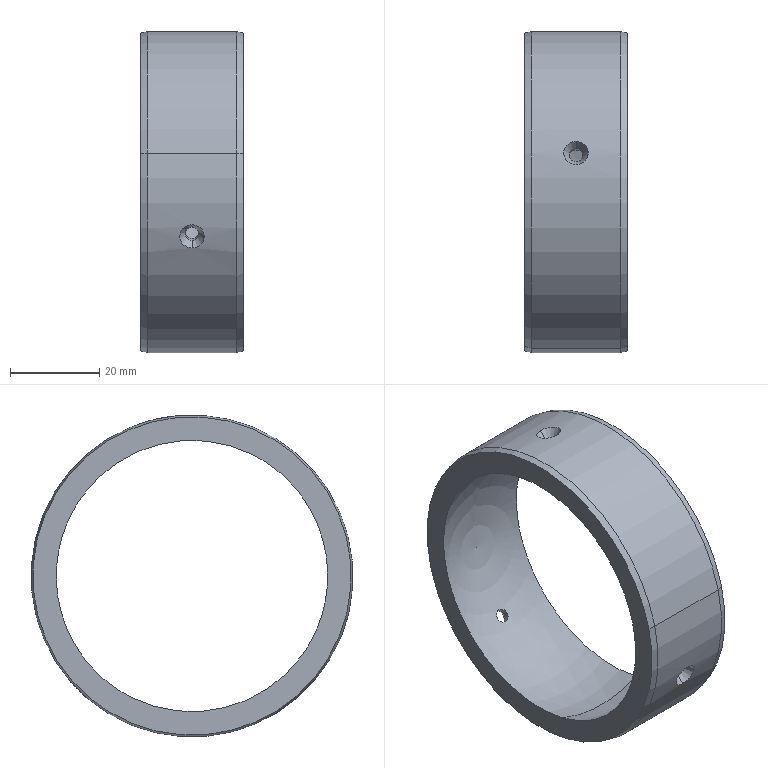Part | SolidWorks | features BaseBody 1 | 1 solid | 22 faces | box 23 x 72 x 72 mm | volume 20485 mm3 | cone 10 | cylinder 8 | sphere 2 | plane 2 | commonest cylinder face diameters 3 x6 72 x2
STEP:
#1=CARTESIAN_POINT('',(272.,34.546,-8.591));
#2=VERTEX_POINT('',#1);
#3=CARTESIAN_POINT('',(272.,-34.546,8.591));
#4=VERTEX_POINT('',#3);
#5=CARTESIAN_POINT('',(272.,0.,0.));
#6=DIRECTION('',(1.,0.,0.));
#7=DIRECTION('',(0.,0.9704,-0.2413));
#8=AXIS2_PLACEMENT_3D('',#5,#6,#7);
#9=CIRCLE('',#8,35.598);
#10=EDGE_CURVE('',#2,#4,#9,.T.);
#11=ORIENTED_EDGE('',*,*,#10,.F.);
#12=CARTESIAN_POINT('',(270.5,34.936,-8.688));
#13=VERTEX_POINT('',#12);
#14=CARTESIAN_POINT('',(272.,34.546,-8.591));
#15=DIRECTION('',(-0.9659,0.2512,-0.06246));
#16=VECTOR('',#15,1000.);
#17=LINE('',#14,#16);
#18=EDGE_CURVE('',#2,#13,#17,.T.);
#19=ORIENTED_EDGE('',*,*,#18,.T.);
#20=CARTESIAN_POINT('',(270.5,-34.936,8.688));
#21=VERTEX_POINT('',#20);
#22=CARTESIAN_POINT('',(270.5,0.,0.));
#23=DIRECTION('',(-1.,0.,0.));
#24=DIRECTION('',(0.,0.9704,-0.2413));
#25=AXIS2_PLACEMENT_3D('',#22,#23,#24);
#26=CIRCLE('',#25,36.);
#27=EDGE_CURVE('',#21,#13,#26,.T.);
#28=ORIENTED_EDGE('',*,*,#27,.F.);
#29=CARTESIAN_POINT('',(272.,-34.546,8.591));
#30=DIRECTION('',(-0.9659,-0.2512,0.06246));
#31=VECTOR('',#30,1000.);
#32=LINE('',#29,#31);
#33=EDGE_CURVE('',#4,#21,#32,.T.);
#34=ORIENTED_EDGE('',*,*,#33,.F.);
#35=EDGE_LOOP('',(#11,#19,#28,#34));
#36=FACE_OUTER_BOUND('',#35,.T.);
#37=CARTESIAN_POINT('',(272.,0.,0.));
#38=DIRECTION('',(-1.,0.,0.));
#39=DIRECTION('',(0.,-0.9704,0.2413));
#40=AXIS2_PLACEMENT_3D('',#37,#38,#39);
#41=CONICAL_SURFACE('',#40,35.598,0.2618);
#42=ADVANCED_FACE('',(#36),#41,.T.);
#43=CARTESIAN_POINT('',(249.,-34.546,8.591));
#44=VERTEX_POINT('',#43);
#45=CARTESIAN_POINT('',(249.,34.546,-8.591));
#46=VERTEX_POINT('',#45);
#47=CARTESIAN_POINT('',(249.,0.,0.));
#48=DIRECTION('',(-1.,0.,0.));
#49=DIRECTION('',(0.,-0.9704,0.2413));
#50=AXIS2_PLACEMENT_3D('',#47,#48,#49);
#51=CIRCLE('',#50,35.598);
#52=EDGE_CURVE('',#44,#46,#51,.T.);
#53=ORIENTED_EDGE('',*,*,#52,.F.);
#54=CARTESIAN_POINT('',(250.5,-34.936,8.688));
#55=VERTEX_POINT('',#54);
#56=CARTESIAN_POINT('',(250.5,-34.936,8.688));
#57=DIRECTION('',(0.9659,-0.2512,0.06246));
#58=VECTOR('',#57,1000.);
#59=LINE('',#56,#58);
#60=EDGE_CURVE('',#44,#55,#59,.T.);
#61=ORIENTED_EDGE('',*,*,#60,.T.);
#62=CARTESIAN_POINT('',(250.5,34.936,-8.688));
#63=VERTEX_POINT('',#62);
#64=CARTESIAN_POINT('',(250.5,0.,0.));
#65=DIRECTION('',(1.,0.,0.));
#66=DIRECTION('',(0.,-0.9704,0.2413));
#67=AXIS2_PLACEMENT_3D('',#64,#65,#66);
#68=CIRCLE('',#67,36.);
#69=EDGE_CURVE('',#63,#55,#68,.T.);
#70=ORIENTED_EDGE('',*,*,#69,.F.);
#71=CARTESIAN_POINT('',(250.5,34.936,-8.688));
#72=DIRECTION('',(0.9659,0.2512,-0.06246));
#73=VECTOR('',#72,1000.);
#74=LINE('',#71,#73);
#75=EDGE_CURVE('',#46,#63,#74,.T.);
#76=ORIENTED_EDGE('',*,*,#75,.F.);
#77=EDGE_LOOP('',(#53,#61,#70,#76));
#78=FACE_OUTER_BOUND('',#77,.T.);
#79=CARTESIAN_POINT('',(250.5,0.,0.));
#80=DIRECTION('',(1.,0.,0.));
#81=DIRECTION('',(0.,0.9704,-0.2413));
#82=AXIS2_PLACEMENT_3D('',#79,#80,#81);
#83=CONICAL_SURFACE('',#82,36.,0.2618);
#84=ADVANCED_FACE('',(#78),#83,.T.);
#85=CARTESIAN_POINT('',(260.5,-32.933,-7.904));
#86=VERTEX_POINT('',#85);
#87=CARTESIAN_POINT('',(260.5,-32.104,-10.787));
#88=VERTEX_POINT('',#87);
#89=CARTESIAN_POINT('',(260.5,-32.519,-9.346));
#90=DIRECTION('',(0.,0.9611,0.2762));
#91=DIRECTION('',(0.,0.2762,-0.9611));
#92=AXIS2_PLACEMENT_3D('',#89,#90,#91);
#93=CIRCLE('',#92,1.5);
#94=EDGE_CURVE('',#86,#88,#93,.T.);
#95=ORIENTED_EDGE('',*,*,#94,.T.);
#96=CARTESIAN_POINT('',(260.5,-33.759,-12.503));
#97=VERTEX_POINT('',#96);
#98=CARTESIAN_POINT('',(260.5,-33.84,-12.587));
#99=DIRECTION('',(0.,-0.6942,-0.7198));
#100=VECTOR('',#99,1000.);
#101=LINE('',#98,#100);
#102=EDGE_CURVE('',#88,#97,#101,.T.);
#103=ORIENTED_EDGE('',*,*,#102,.T.);
#104=CARTESIAN_POINT('',(260.5,-35.246,-7.329));
#105=VERTEX_POINT('',#104);
#106=CARTESIAN_POINT('',(260.5,-35.246,-7.329));
#107=CARTESIAN_POINT('',(260.68,-35.246,-7.329));
#108=CARTESIAN_POINT('',(260.856,-35.243,-7.345));
#109=CARTESIAN_POINT('',(261.204,-35.229,-7.411));
#110=CARTESIAN_POINT('',(261.378,-35.218,-7.461));
#111=CARTESIAN_POINT('',(261.709,-35.191,-7.591));
#112=CARTESIAN_POINT('',(261.866,-35.173,-7.671));
#113=CARTESIAN_POINT('',(262.164,-35.132,-7.86));
#114=CARTESIAN_POINT('',(262.306,-35.107,-7.97));
#115=CARTESIAN_POINT('',(262.561,-35.051,-8.211));
#116=CARTESIAN_POINT('',(262.676,-35.02,-8.342));
#117=CARTESIAN_POINT('',(262.879,-34.951,-8.628));
#118=CARTESIAN_POINT('',(262.966,-34.913,-8.781));
#119=CARTESIAN_POINT('',(263.175,-34.792,-9.254));
#120=CARTESIAN_POINT('',(263.25,-34.698,-9.6));
#121=CARTESIAN_POINT('',(263.25,-34.551,-10.111));
#122=CARTESIAN_POINT('',(263.232,-34.5,-10.284));
#123=CARTESIAN_POINT('',(263.161,-34.399,-10.618));
#124=CARTESIAN_POINT('',(263.108,-34.349,-10.78));
#125=CARTESIAN_POINT('',(262.968,-34.249,-11.092));
#126=CARTESIAN_POINT('',(262.88,-34.2,-11.243));
#127=CARTESIAN_POINT('',(262.679,-34.107,-11.52));
#128=CARTESIAN_POINT('',(262.564,-34.063,-11.649));
#129=CARTESIAN_POINT('',(262.178,-33.941,-12.004));
#130=CARTESIAN_POINT('',(261.871,-33.874,-12.19));
#131=CARTESIAN_POINT('',(261.378,-33.806,-12.376));
#132=CARTESIAN_POINT('',(261.205,-33.788,-12.424));
#133=CARTESIAN_POINT('',(260.854,-33.765,-12.487));
#134=CARTESIAN_POINT('',(260.678,-33.759,-12.503));
#135=CARTESIAN_POINT('',(260.5,-33.759,-12.503));
#136=B_SPLINE_CURVE_WITH_KNOTS('',3,(#106,#107,#108,#109,#110,#111,#112,#113,#114,#115,#116,#117,#118,#119,#120,#121,#122,#123,#124,#125,#126,#127,#128,#129,#130,#131,#132,#133,#134,#135),.UNSPECIFIED.,.F.,.F.,(4,2,2,2,2,2,2,2,2,2,2,2,2,2,4),(0.01008,0.01062,0.01115,0.01168,0.01221,0.01274,0.01328,0.01434,0.01487,0.0154,0.01594,0.01647,0.01753,0.01806,0.0186),.UNSPECIFIED.);
#137=EDGE_CURVE('',#105,#97,#136,.T.);
#138=ORIENTED_EDGE('',*,*,#137,.F.);
#139=CARTESIAN_POINT('',(260.5,-35.359,-7.301));
#140=DIRECTION('',(0.,-0.9704,0.2413));
#141=VECTOR('',#140,1000.);
#142=LINE('',#139,#141);
#143=EDGE_CURVE('',#86,#105,#142,.T.);
#144=ORIENTED_EDGE('',*,*,#143,.F.);
#145=EDGE_LOOP('',(#95,#103,#138,#144));
#146=FACE_OUTER_BOUND('',#145,.T.);
#147=CARTESIAN_POINT('',(260.5,-34.599,-9.944));
#148=DIRECTION('',(0.,-0.9611,-0.2762));
#149=DIRECTION('',(0.,-0.2762,0.9611));
#150=AXIS2_PLACEMENT_3D('',#147,#148,#149);
#151=CONICAL_SURFACE('',#150,2.75,0.5236);
#152=ADVANCED_FACE('',(#146),#151,.F.);
#153=ORIENTED_EDGE('',*,*,#94,.F.);
#154=CARTESIAN_POINT('',(260.5,-31.569,-7.512));
#155=VERTEX_POINT('',#154);
#156=CARTESIAN_POINT('',(260.5,-0.4143,1.442));
#157=DIRECTION('',(0.,0.9611,0.2762));
#158=VECTOR('',#157,1000.);
#159=LINE('',#156,#158);
#160=EDGE_CURVE('',#86,#155,#159,.T.);
#161=ORIENTED_EDGE('',*,*,#160,.T.);
#162=CARTESIAN_POINT('',(260.5,-30.74,-10.395));
#163=VERTEX_POINT('',#162);
#164=CARTESIAN_POINT('',(260.5,-31.154,-8.954));
#165=DIRECTION('',(0.,-0.9611,-0.2762));
#166=DIRECTION('',(0.,0.2762,-0.9611));
#167=AXIS2_PLACEMENT_3D('',#164,#165,#166);
#168=CIRCLE('',#167,1.5);
#169=EDGE_CURVE('',#163,#155,#168,.T.);
#170=ORIENTED_EDGE('',*,*,#169,.F.);
#171=CARTESIAN_POINT('',(260.5,0.4143,-1.442));
#172=DIRECTION('',(0.,0.9611,0.2762));
#173=VECTOR('',#172,1000.);
#174=LINE('',#171,#173);
#175=EDGE_CURVE('',#88,#163,#174,.T.);
#176=ORIENTED_EDGE('',*,*,#175,.F.);
#177=EDGE_LOOP('',(#153,#161,#170,#176));
#178=FACE_OUTER_BOUND('',#177,.T.);
#179=CARTESIAN_POINT('',(260.5,0.,0.));
#180=DIRECTION('',(0.,0.9611,0.2762));
#181=DIRECTION('',(0.,0.2762,-0.9611));
#182=AXIS2_PLACEMENT_3D('',#179,#180,#181);
#183=CYLINDRICAL_SURFACE('',#182,1.5);
#184=ADVANCED_FACE('',(#178),#183,.F.);
#185=CARTESIAN_POINT('',(260.5,23.312,-24.569));
#186=VERTEX_POINT('',#185);
#187=CARTESIAN_POINT('',(260.5,25.394,-22.41));
#188=VERTEX_POINT('',#187);
#189=CARTESIAN_POINT('',(260.5,24.353,-23.489));
#190=DIRECTION('',(0.,-0.7198,0.6942));
#191=DIRECTION('',(0.,0.6942,0.7198));
#192=AXIS2_PLACEMENT_3D('',#189,#190,#191);
#193=CIRCLE('',#192,1.5);
#194=EDGE_CURVE('',#186,#188,#193,.T.);
#195=ORIENTED_EDGE('',*,*,#194,.T.);
#196=CARTESIAN_POINT('',(260.5,27.707,-22.985));
#197=VERTEX_POINT('',#196);
#198=CARTESIAN_POINT('',(260.5,27.82,-23.013));
#199=DIRECTION('',(0.,0.9704,-0.2413));
#200=VECTOR('',#199,1000.);
#201=LINE('',#198,#200);
#202=EDGE_CURVE('',#188,#197,#201,.T.);
#203=ORIENTED_EDGE('',*,*,#202,.T.);
#204=CARTESIAN_POINT('',(260.5,23.97,-26.86));
#205=VERTEX_POINT('',#204);
#206=CARTESIAN_POINT('',(260.5,23.97,-26.86));
#207=CARTESIAN_POINT('',(260.677,23.97,-26.86));
#208=CARTESIAN_POINT('',(260.858,23.983,-26.848));
#209=CARTESIAN_POINT('',(261.207,24.033,-26.803));
#210=CARTESIAN_POINT('',(261.377,24.071,-26.77));
#211=CARTESIAN_POINT('',(261.707,24.169,-26.681));
#212=CARTESIAN_POINT('',(261.868,24.231,-26.625));
#213=CARTESIAN_POINT('',(262.166,24.373,-26.494));
#214=CARTESIAN_POINT('',(262.304,24.454,-26.42));
#215=CARTESIAN_POINT('',(262.69,24.728,-26.165));
#216=CARTESIAN_POINT('',(262.895,24.942,-25.962));
#217=CARTESIAN_POINT('',(263.177,25.414,-25.5));
#218=CARTESIAN_POINT('',(263.25,25.665,-25.247));
#219=CARTESIAN_POINT('',(263.25,26.034,-24.865));
#220=CARTESIAN_POINT('',(263.232,26.158,-24.734));
#221=CARTESIAN_POINT('',(263.16,26.397,-24.479));
#222=CARTESIAN_POINT('',(263.107,26.512,-24.355));
#223=CARTESIAN_POINT('',(262.967,26.732,-24.113));
#224=CARTESIAN_POINT('',(262.879,26.838,-23.995));
#225=CARTESIAN_POINT('',(262.678,27.032,-23.776));
#226=CARTESIAN_POINT('',(262.563,27.121,-23.674));
#227=CARTESIAN_POINT('',(262.305,27.285,-23.485));
#228=CARTESIAN_POINT('',(262.166,27.357,-23.401));
#229=CARTESIAN_POINT('',(261.868,27.482,-23.254));
#230=CARTESIAN_POINT('',(261.708,27.536,-23.19));
#231=CARTESIAN_POINT('',(261.377,27.621,-23.089));
#232=CARTESIAN_POINT('',(261.207,27.653,-23.05));
#233=CARTESIAN_POINT('',(260.858,27.696,-22.998));
#234=CARTESIAN_POINT('',(260.677,27.707,-22.985));
#235=CARTESIAN_POINT('',(260.5,27.707,-22.985));
#236=B_SPLINE_CURVE_WITH_KNOTS('',3,(#206,#207,#208,#209,#210,#211,#212,#213,#214,#215,#216,#217,#218,#219,#220,#221,#222,#223,#224,#225,#226,#227,#228,#229,#230,#231,#232,#233,#234,#235),.UNSPECIFIED.,.F.,.F.,(4,2,2,2,2,2,2,2,2,2,2,2,2,2,4),(0.01333,0.01386,0.01439,0.01492,0.01545,0.01652,0.01758,0.01811,0.01864,0.01917,0.0197,0.02023,0.02076,0.02129,0.02182),.UNSPECIFIED.);
#237=EDGE_CURVE('',#205,#197,#236,.T.);
#238=ORIENTED_EDGE('',*,*,#237,.F.);
#239=CARTESIAN_POINT('',(260.5,24.002,-26.972));
#240=DIRECTION('',(0.,0.2762,-0.9611));
#241=VECTOR('',#240,1000.);
#242=LINE('',#239,#241);
#243=EDGE_CURVE('',#186,#205,#242,.T.);
#244=ORIENTED_EDGE('',*,*,#243,.F.);
#245=EDGE_LOOP('',(#195,#203,#238,#244));
#246=FACE_OUTER_BOUND('',#245,.T.);
#247=CARTESIAN_POINT('',(260.5,25.911,-24.992));
#248=DIRECTION('',(0.,0.7198,-0.6942));
#249=DIRECTION('',(0.,-0.6942,-0.7198));
#250=AXIS2_PLACEMENT_3D('',#247,#248,#249);
#251=CONICAL_SURFACE('',#250,2.75,0.5236);
#252=ADVANCED_FACE('',(#246),#251,.F.);
#253=ORIENTED_EDGE('',*,*,#194,.F.);
#254=CARTESIAN_POINT('',(260.5,22.29,-23.583));
#255=VERTEX_POINT('',#254);
#256=CARTESIAN_POINT('',(260.5,-1.041,-1.08));
#257=DIRECTION('',(0.,-0.7198,0.6942));
#258=VECTOR('',#257,1000.);
#259=LINE('',#256,#258);
#260=EDGE_CURVE('',#186,#255,#259,.T.);
#261=ORIENTED_EDGE('',*,*,#260,.T.);
#262=CARTESIAN_POINT('',(260.5,24.372,-21.424));
#263=VERTEX_POINT('',#262);
#264=CARTESIAN_POINT('',(260.5,23.331,-22.504));
#265=DIRECTION('',(0.,0.7198,-0.6942));
#266=DIRECTION('',(0.,0.6942,0.7198));
#267=AXIS2_PLACEMENT_3D('',#264,#265,#266);
#268=CIRCLE('',#267,1.5);
#269=EDGE_CURVE('',#263,#255,#268,.T.);
#270=ORIENTED_EDGE('',*,*,#269,.F.);
#271=CARTESIAN_POINT('',(260.5,1.041,1.08));
#272=DIRECTION('',(0.,-0.7198,0.6942));
#273=VECTOR('',#272,1000.);
#274=LINE('',#271,#273);
#275=EDGE_CURVE('',#188,#263,#274,.T.);
#276=ORIENTED_EDGE('',*,*,#275,.F.);
#277=EDGE_LOOP('',(#253,#261,#270,#276));
#278=FACE_OUTER_BOUND('',#277,.T.);
#279=CARTESIAN_POINT('',(260.5,0.,0.));
#280=DIRECTION('',(0.,-0.7198,0.6942));
#281=DIRECTION('',(0.,0.6942,0.7198));
#282=AXIS2_PLACEMENT_3D('',#279,#280,#281);
#283=CYLINDRICAL_SURFACE('',#282,1.5);
#284=ADVANCED_FACE('',(#278),#283,.F.);
#285=CARTESIAN_POINT('',(260.5,9.621,32.473));
#286=VERTEX_POINT('',#285);
#287=CARTESIAN_POINT('',(260.5,6.71,33.197));
#288=VERTEX_POINT('',#287);
#289=CARTESIAN_POINT('',(260.5,8.166,32.835));
#290=DIRECTION('',(0.,-0.2413,-0.9704));
#291=DIRECTION('',(0.,-0.9704,0.2413));
#292=AXIS2_PLACEMENT_3D('',#289,#290,#291);
#293=CIRCLE('',#292,1.5);
#294=EDGE_CURVE('',#286,#288,#293,.T.);
#295=ORIENTED_EDGE('',*,*,#294,.T.);
#296=CARTESIAN_POINT('',(260.5,6.052,35.488));
#297=VERTEX_POINT('',#296);
#298=CARTESIAN_POINT('',(260.5,6.02,35.6));
#299=DIRECTION('',(0.,-0.2762,0.9611));
#300=VECTOR('',#299,1000.);
#301=LINE('',#298,#300);
#302=EDGE_CURVE('',#288,#297,#301,.T.);
#303=ORIENTED_EDGE('',*,*,#302,.T.);
#304=CARTESIAN_POINT('',(260.5,11.276,34.188));
#305=VERTEX_POINT('',#304);
#306=CARTESIAN_POINT('',(260.5,11.276,34.188));
#307=CARTESIAN_POINT('',(260.855,11.276,34.188));
#308=CARTESIAN_POINT('',(261.213,11.211,34.21));
#309=CARTESIAN_POINT('',(261.871,10.959,34.292));
#310=CARTESIAN_POINT('',(262.178,10.771,34.352));
#311=CARTESIAN_POINT('',(262.564,10.412,34.462));
#312=CARTESIAN_POINT('',(262.679,10.282,34.501));
#313=CARTESIAN_POINT('',(262.88,10.002,34.583));
#314=CARTESIAN_POINT('',(262.967,9.85,34.627));
#315=CARTESIAN_POINT('',(263.107,9.534,34.715));
#316=CARTESIAN_POINT('',(263.16,9.371,34.759));
#317=CARTESIAN_POINT('',(263.232,9.034,34.848));
#318=CARTESIAN_POINT('',(263.25,8.86,34.893));
#319=CARTESIAN_POINT('',(263.25,8.343,35.022));
#320=CARTESIAN_POINT('',(263.176,7.994,35.103));
#321=CARTESIAN_POINT('',(262.967,7.516,35.207));
#322=CARTESIAN_POINT('',(262.88,7.362,35.24));
#323=CARTESIAN_POINT('',(262.677,7.074,35.298));
#324=CARTESIAN_POINT('',(262.562,6.941,35.325));
#325=CARTESIAN_POINT('',(262.307,6.698,35.372));
#326=CARTESIAN_POINT('',(262.165,6.587,35.392));
#327=CARTESIAN_POINT('',(261.867,6.397,35.427));
#328=CARTESIAN_POINT('',(261.71,6.317,35.442));
#329=CARTESIAN_POINT('',(261.211,6.119,35.476));
#330=CARTESIAN_POINT('',(260.858,6.052,35.488));
#331=CARTESIAN_POINT('',(260.5,6.052,35.488));
#332=B_SPLINE_CURVE_WITH_KNOTS('',3,(#306,#307,#308,#309,#310,#311,#312,#313,#314,#315,#316,#317,#318,#319,#320,#321,#322,#323,#324,#325,#326,#327,#328,#329,#330,#331),.UNSPECIFIED.,.F.,.F.,(4,2,2,2,2,2,2,2,2,2,2,2,4),(0.01491,0.01597,0.01704,0.01757,0.0181,0.01863,0.01916,0.02023,0.02076,0.02129,0.02182,0.02235,0.02341),.UNSPECIFIED.);
#333=EDGE_CURVE('',#305,#297,#332,.T.);
#334=ORIENTED_EDGE('',*,*,#333,.F.);
#335=CARTESIAN_POINT('',(260.5,11.357,34.272));
#336=DIRECTION('',(0.,0.6942,0.7198));
#337=VECTOR('',#336,1000.);
#338=LINE('',#335,#337);
#339=EDGE_CURVE('',#286,#305,#338,.T.);
#340=ORIENTED_EDGE('',*,*,#339,.F.);
#341=EDGE_LOOP('',(#295,#303,#334,#340));
#342=FACE_OUTER_BOUND('',#341,.T.);
#343=CARTESIAN_POINT('',(260.5,8.688,34.936));
#344=DIRECTION('',(0.,0.2413,0.9704));
#345=DIRECTION('',(0.,0.9704,-0.2413));
#346=AXIS2_PLACEMENT_3D('',#343,#344,#345);
#347=CONICAL_SURFACE('',#346,2.75,0.5236);
#348=ADVANCED_FACE('',(#342),#347,.F.);
#349=ORIENTED_EDGE('',*,*,#294,.F.);
#350=CARTESIAN_POINT('',(260.5,9.279,31.095));
#351=VERTEX_POINT('',#350);
#352=CARTESIAN_POINT('',(260.5,1.456,-0.362));
#353=DIRECTION('',(0.,-0.2413,-0.9704));
#354=VECTOR('',#353,1000.);
#355=LINE('',#352,#354);
#356=EDGE_CURVE('',#286,#351,#355,.T.);
#357=ORIENTED_EDGE('',*,*,#356,.T.);
#358=CARTESIAN_POINT('',(262.,7.823,31.457));
#359=VERTEX_POINT('',#358);
#360=CARTESIAN_POINT('',(260.5,7.823,31.457));
#361=DIRECTION('',(0.,0.2413,0.9704));
#362=DIRECTION('',(0.,-0.9704,0.2413));
#363=AXIS2_PLACEMENT_3D('',#360,#361,#362);
#364=CIRCLE('',#363,1.5);
#365=EDGE_CURVE('',#359,#351,#364,.T.);
#366=ORIENTED_EDGE('',*,*,#365,.F.);
#367=CARTESIAN_POINT('',(260.5,6.367,31.819));
#368=VERTEX_POINT('',#367);
#369=CARTESIAN_POINT('',(260.5,7.823,31.457));
#370=DIRECTION('',(0.,0.2413,0.9704));
#371=DIRECTION('',(0.,-0.9704,0.2413));
#372=AXIS2_PLACEMENT_3D('',#369,#370,#371);
#373=CIRCLE('',#372,1.5);
#374=EDGE_CURVE('',#368,#359,#373,.T.);
#375=ORIENTED_EDGE('',*,*,#374,.F.);
#376=CARTESIAN_POINT('',(260.5,-1.456,0.362));
#377=DIRECTION('',(0.,-0.2413,-0.9704));
#378=VECTOR('',#377,1000.);
#379=LINE('',#376,#378);
#380=EDGE_CURVE('',#288,#368,#379,.T.);
#381=ORIENTED_EDGE('',*,*,#380,.F.);
#382=EDGE_LOOP('',(#349,#357,#366,#375,#381));
#383=FACE_OUTER_BOUND('',#382,.T.);
#384=CARTESIAN_POINT('',(260.5,0.,0.));
#385=DIRECTION('',(0.,-0.2413,-0.9704));
#386=DIRECTION('',(0.,-0.9704,0.2413));
#387=AXIS2_PLACEMENT_3D('',#384,#385,#386);
#388=CYLINDRICAL_SURFACE('',#387,1.5);
#389=ADVANCED_FACE('',(#383),#388,.F.);
#390=ORIENTED_EDGE('',*,*,#333,.T.);
#391=CARTESIAN_POINT('',(260.5,6.052,35.488));
#392=CARTESIAN_POINT('',(260.321,6.052,35.488));
#393=CARTESIAN_POINT('',(260.144,6.068,35.485));
#394=CARTESIAN_POINT('',(259.796,6.135,35.473));
#395=CARTESIAN_POINT('',(259.622,6.185,35.465));
#396=CARTESIAN_POINT('',(259.292,6.316,35.442));
#397=CARTESIAN_POINT('',(259.134,6.396,35.427));
#398=CARTESIAN_POINT('',(258.836,6.587,35.392));
#399=CARTESIAN_POINT('',(258.694,6.697,35.372));
#400=CARTESIAN_POINT('',(258.439,6.94,35.325));
#401=CARTESIAN_POINT('',(258.324,7.073,35.299));
#402=CARTESIAN_POINT('',(258.121,7.361,35.24));
#403=CARTESIAN_POINT('',(258.034,7.515,35.207));
#404=CARTESIAN_POINT('',(257.894,7.833,35.138));
#405=CARTESIAN_POINT('',(257.84,8.,35.1));
#406=CARTESIAN_POINT('',(257.768,8.342,35.021));
#407=CARTESIAN_POINT('',(257.75,8.514,34.979));
#408=CARTESIAN_POINT('',(257.75,8.858,34.894));
#409=CARTESIAN_POINT('',(257.768,9.033,34.849));
#410=CARTESIAN_POINT('',(257.84,9.37,34.76));
#411=CARTESIAN_POINT('',(257.893,9.534,34.715));
#412=CARTESIAN_POINT('',(258.103,10.009,34.582));
#413=CARTESIAN_POINT('',(258.309,10.294,34.498));
#414=CARTESIAN_POINT('',(258.694,10.652,34.388));
#415=CARTESIAN_POINT('',(258.833,10.757,34.355));
#416=CARTESIAN_POINT('',(259.131,10.942,34.297));
#417=CARTESIAN_POINT('',(259.292,11.021,34.271));
#418=CARTESIAN_POINT('',(259.622,11.148,34.231));
#419=CARTESIAN_POINT('',(259.792,11.195,34.215));
#420=CARTESIAN_POINT('',(260.143,11.26,34.194));
#421=CARTESIAN_POINT('',(260.323,11.276,34.188));
#422=CARTESIAN_POINT('',(260.5,11.276,34.188));
#423=B_SPLINE_CURVE_WITH_KNOTS('',3,(#391,#392,#393,#394,#395,#396,#397,#398,#399,#400,#401,#402,#403,#404,#405,#406,#407,#408,#409,#410,#411,#412,#413,#414,#415,#416,#417,#418,#419,#420,#421,#422),.UNSPECIFIED.,.F.,.F.,(4,2,2,2,2,2,2,2,2,2,2,2,2,2,2,4),(0.006404,0.006936,0.007468,0.007999,0.008531,0.009063,0.009594,0.01013,0.01066,0.01119,0.01172,0.01278,0.01332,0.01385,0.01438,0.01491),.UNSPECIFIED.);
#424=EDGE_CURVE('',#297,#305,#423,.T.);
#425=ORIENTED_EDGE('',*,*,#424,.T.);
#426=EDGE_LOOP('',(#390,#425));
#427=FACE_BOUND('',#426,.T.);
#428=ORIENTED_EDGE('',*,*,#69,.T.);
#429=CARTESIAN_POINT('',(260.5,-34.936,8.688));
#430=DIRECTION('',(1.,0.,0.));
#431=VECTOR('',#430,1000.);
#432=LINE('',#429,#431);
#433=EDGE_CURVE('',#55,#21,#432,.T.);
#434=ORIENTED_EDGE('',*,*,#433,.T.);
#435=ORIENTED_EDGE('',*,*,#27,.T.);
#436=CARTESIAN_POINT('',(260.5,34.936,-8.688));
#437=DIRECTION('',(1.,0.,0.));
#438=VECTOR('',#437,1000.);
#439=LINE('',#436,#438);
#440=EDGE_CURVE('',#63,#13,#439,.T.);
#441=ORIENTED_EDGE('',*,*,#440,.F.);
#442=EDGE_LOOP('',(#428,#434,#435,#441));
#443=FACE_OUTER_BOUND('',#442,.T.);
#444=CARTESIAN_POINT('',(260.5,0.,0.));
#445=DIRECTION('',(1.,0.,0.));
#446=DIRECTION('',(0.,0.9704,-0.2413));
#447=AXIS2_PLACEMENT_3D('',#444,#445,#446);
#448=CYLINDRICAL_SURFACE('',#447,36.);
#449=ADVANCED_FACE('',(#427,#443),#448,.T.);
#450=ORIENTED_EDGE('',*,*,#269,.T.);
#451=CARTESIAN_POINT('',(260.5,23.331,-22.504));
#452=DIRECTION('',(0.,0.7198,-0.6942));
#453=DIRECTION('',(0.,0.6942,0.7198));
#454=AXIS2_PLACEMENT_3D('',#451,#452,#453);
#455=CIRCLE('',#454,1.5);
#456=EDGE_CURVE('',#255,#263,#455,.T.);
#457=ORIENTED_EDGE('',*,*,#456,.T.);
#458=EDGE_LOOP('',(#450,#457));
#459=FACE_BOUND('',#458,.T.);
#460=CARTESIAN_POINT('',(249.,-7.323,-29.447));
#461=VERTEX_POINT('',#460);
#462=CARTESIAN_POINT('',(249.,7.323,29.447));
#463=VERTEX_POINT('',#462);
#464=CARTESIAN_POINT('',(249.,0.,0.));
#465=DIRECTION('',(1.,0.,0.));
#466=DIRECTION('',(0.,0.9704,-0.2413));
#467=AXIS2_PLACEMENT_3D('',#464,#465,#466);
#468=CIRCLE('',#467,30.344);
#469=EDGE_CURVE('',#461,#463,#468,.T.);
#470=ORIENTED_EDGE('',*,*,#469,.F.);
#471=CARTESIAN_POINT('',(272.,-7.323,-29.447));
#472=VERTEX_POINT('',#471);
#473=CARTESIAN_POINT('',(260.5,0.,0.));
#474=DIRECTION('',(0.,-0.9704,0.2413));
#475=DIRECTION('',(0.,-0.2413,-0.9704));
#476=AXIS2_PLACEMENT_3D('',#473,#474,#475);
#477=CIRCLE('',#476,32.45);
#478=EDGE_CURVE('',#461,#472,#477,.T.);
#479=ORIENTED_EDGE('',*,*,#478,.T.);
#480=CARTESIAN_POINT('',(272.,7.323,29.447));
#481=VERTEX_POINT('',#480);
#482=CARTESIAN_POINT('',(272.,0.,0.));
#483=DIRECTION('',(1.,0.,0.));
#484=DIRECTION('',(0.,0.9704,-0.2413));
#485=AXIS2_PLACEMENT_3D('',#482,#483,#484);
#486=CIRCLE('',#485,30.344);
#487=EDGE_CURVE('',#472,#481,#486,.T.);
#488=ORIENTED_EDGE('',*,*,#487,.T.);
#489=CARTESIAN_POINT('',(260.5,0.,0.));
#490=DIRECTION('',(0.,0.9704,-0.2413));
#491=DIRECTION('',(0.,0.2413,0.9704));
#492=AXIS2_PLACEMENT_3D('',#489,#490,#491);
#493=CIRCLE('',#492,32.45);
#494=EDGE_CURVE('',#359,#481,#493,.T.);
#495=ORIENTED_EDGE('',*,*,#494,.F.);
#496=ORIENTED_EDGE('',*,*,#365,.T.);
#497=CARTESIAN_POINT('',(259.,7.823,31.457));
#498=VERTEX_POINT('',#497);
#499=CARTESIAN_POINT('',(260.5,7.823,31.457));
#500=DIRECTION('',(0.,0.2413,0.9704));
#501=DIRECTION('',(0.,-0.9704,0.2413));
#502=AXIS2_PLACEMENT_3D('',#499,#500,#501);
#503=CIRCLE('',#502,1.5);
#504=EDGE_CURVE('',#351,#498,#503,.T.);
#505=ORIENTED_EDGE('',*,*,#504,.T.);
#506=CARTESIAN_POINT('',(260.5,0.,0.));
#507=DIRECTION('',(0.,0.9704,-0.2413));
#508=DIRECTION('',(0.,0.2413,0.9704));
#509=AXIS2_PLACEMENT_3D('',#506,#507,#508);
#510=CIRCLE('',#509,32.45);
#511=EDGE_CURVE('',#463,#498,#510,.T.);
#512=ORIENTED_EDGE('',*,*,#511,.F.);
#513=EDGE_LOOP('',(#470,#479,#488,#495,#496,#505,#512));
#514=FACE_OUTER_BOUND('',#513,.T.);
#515=CARTESIAN_POINT('',(260.5,0.,0.));
#516=DIRECTION('',(0.,-0.9704,0.2413));
#517=DIRECTION('',(0.,0.2413,0.9704));
#518=AXIS2_PLACEMENT_3D('',#515,#516,#517);
#519=SPHERICAL_SURFACE('',#518,32.45);
#520=ADVANCED_FACE('',(#459,#514),#519,.F.);
#521=ORIENTED_EDGE('',*,*,#478,.F.);
#522=CARTESIAN_POINT('',(249.,0.,0.));
#523=DIRECTION('',(1.,0.,0.));
#524=DIRECTION('',(0.,0.9704,-0.2413));
#525=AXIS2_PLACEMENT_3D('',#522,#523,#524);
#526=CIRCLE('',#525,30.344);
#527=EDGE_CURVE('',#463,#461,#526,.T.);
#528=ORIENTED_EDGE('',*,*,#527,.F.);
#529=ORIENTED_EDGE('',*,*,#511,.T.);
#530=CARTESIAN_POINT('',(260.5,7.823,31.457));
#531=DIRECTION('',(0.,0.2413,0.9704));
#532=DIRECTION('',(0.,-0.9704,0.2413));
#533=AXIS2_PLACEMENT_3D('',#530,#531,#532);
#534=CIRCLE('',#533,1.5);
#535=EDGE_CURVE('',#498,#368,#534,.T.);
#536=ORIENTED_EDGE('',*,*,#535,.T.);
#537=ORIENTED_EDGE('',*,*,#374,.T.);
#538=ORIENTED_EDGE('',*,*,#494,.T.);
#539=CARTESIAN_POINT('',(272.,0.,0.));
#540=DIRECTION('',(1.,0.,0.));
#541=DIRECTION('',(0.,0.9704,-0.2413));
#542=AXIS2_PLACEMENT_3D('',#539,#540,#541);
#543=CIRCLE('',#542,30.344);
#544=EDGE_CURVE('',#481,#472,#543,.T.);
#545=ORIENTED_EDGE('',*,*,#544,.T.);
#546=EDGE_LOOP('',(#521,#528,#529,#536,#537,#538,#545));
#547=FACE_OUTER_BOUND('',#546,.T.);
#548=ORIENTED_EDGE('',*,*,#169,.T.);
#549=CARTESIAN_POINT('',(260.5,-31.154,-8.954));
#550=DIRECTION('',(0.,-0.9611,-0.2762));
#551=DIRECTION('',(0.,0.2762,-0.9611));
#552=AXIS2_PLACEMENT_3D('',#549,#550,#551);
#553=CIRCLE('',#552,1.5);
#554=EDGE_CURVE('',#155,#163,#553,.T.);
#555=ORIENTED_EDGE('',*,*,#554,.T.);
#556=EDGE_LOOP('',(#548,#555));
#557=FACE_BOUND('',#556,.T.);
#558=CARTESIAN_POINT('',(260.5,0.,0.));
#559=DIRECTION('',(0.,-0.9704,0.2413));
#560=DIRECTION('',(0.,0.2413,0.9704));
#561=AXIS2_PLACEMENT_3D('',#558,#559,#560);
#562=SPHERICAL_SURFACE('',#561,32.45);
#563=ADVANCED_FACE('',(#547,#557),#562,.F.);
#564=ORIENTED_EDGE('',*,*,#433,.F.);
#565=CARTESIAN_POINT('',(250.5,0.,0.));
#566=DIRECTION('',(1.,0.,0.));
#567=DIRECTION('',(0.,-0.9704,0.2413));
#568=AXIS2_PLACEMENT_3D('',#565,#566,#567);
#569=CIRCLE('',#568,36.);
#570=EDGE_CURVE('',#55,#63,#569,.T.);
#571=ORIENTED_EDGE('',*,*,#570,.T.);
#572=ORIENTED_EDGE('',*,*,#440,.T.);
#573=CARTESIAN_POINT('',(270.5,0.,0.));
#574=DIRECTION('',(-1.,0.,0.));
#575=DIRECTION('',(0.,0.9704,-0.2413));
#576=AXIS2_PLACEMENT_3D('',#573,#574,#575);
#577=CIRCLE('',#576,36.);
#578=EDGE_CURVE('',#13,#21,#577,.T.);
#579=ORIENTED_EDGE('',*,*,#578,.T.);
#580=EDGE_LOOP('',(#564,#571,#572,#579));
#581=FACE_OUTER_BOUND('',#580,.T.);
#582=ORIENTED_EDGE('',*,*,#237,.T.);
#583=CARTESIAN_POINT('',(260.5,27.707,-22.985));
#584=CARTESIAN_POINT('',(260.322,27.707,-22.985));
#585=CARTESIAN_POINT('',(260.146,27.697,-22.998));
#586=CARTESIAN_POINT('',(259.795,27.653,-23.05));
#587=CARTESIAN_POINT('',(259.622,27.621,-23.089));
#588=CARTESIAN_POINT('',(259.129,27.493,-23.241));
#589=CARTESIAN_POINT('',(258.822,27.365,-23.392));
#590=CARTESIAN_POINT('',(258.44,27.123,-23.672));
#591=CARTESIAN_POINT('',(258.323,27.032,-23.776));
#592=CARTESIAN_POINT('',(258.12,26.837,-23.996));
#593=CARTESIAN_POINT('',(258.034,26.734,-24.111));
#594=CARTESIAN_POINT('',(257.894,26.513,-24.353));
#595=CARTESIAN_POINT('',(257.84,26.396,-24.48));
#596=CARTESIAN_POINT('',(257.768,26.158,-24.734));
#597=CARTESIAN_POINT('',(257.75,26.037,-24.862));
#598=CARTESIAN_POINT('',(257.75,25.788,-25.12));
#599=CARTESIAN_POINT('',(257.768,25.663,-25.247));
#600=CARTESIAN_POINT('',(257.839,25.418,-25.494));
#601=CARTESIAN_POINT('',(257.893,25.296,-25.615));
#602=CARTESIAN_POINT('',(258.034,25.061,-25.845));
#603=CARTESIAN_POINT('',(258.12,24.949,-25.953));
#604=CARTESIAN_POINT('',(258.322,24.737,-26.155));
#605=CARTESIAN_POINT('',(258.439,24.636,-26.25));
#606=CARTESIAN_POINT('',(258.694,24.455,-26.419));
#607=CARTESIAN_POINT('',(258.833,24.374,-26.494));
#608=CARTESIAN_POINT('',(259.133,24.23,-26.625));
#609=CARTESIAN_POINT('',(259.293,24.169,-26.681));
#610=CARTESIAN_POINT('',(259.622,24.071,-26.769));
#611=CARTESIAN_POINT('',(259.794,24.033,-26.803));
#612=CARTESIAN_POINT('',(260.146,23.982,-26.849));
#613=CARTESIAN_POINT('',(260.322,23.97,-26.86));
#614=CARTESIAN_POINT('',(260.5,23.97,-26.86));
#615=B_SPLINE_CURVE_WITH_KNOTS('',3,(#583,#584,#585,#586,#587,#588,#589,#590,#591,#592,#593,#594,#595,#596,#597,#598,#599,#600,#601,#602,#603,#604,#605,#606,#607,#608,#609,#610,#611,#612,#613,#614),.UNSPECIFIED.,.F.,.F.,(4,2,2,2,2,2,2,2,2,2,2,2,2,2,2,4),(0.004829,0.00536,0.005892,0.006954,0.007486,0.008017,0.008548,0.009079,0.009611,0.01014,0.01067,0.0112,0.01174,0.01227,0.0128,0.01333),.UNSPECIFIED.);
#616=EDGE_CURVE('',#197,#205,#615,.T.);
#617=ORIENTED_EDGE('',*,*,#616,.T.);
#618=EDGE_LOOP('',(#582,#617));
#619=FACE_BOUND('',#618,.T.);
#620=ORIENTED_EDGE('',*,*,#137,.T.);
#621=CARTESIAN_POINT('',(260.5,-33.759,-12.503));
#622=CARTESIAN_POINT('',(260.322,-33.759,-12.503));
#623=CARTESIAN_POINT('',(260.142,-33.765,-12.487));
#624=CARTESIAN_POINT('',(259.793,-33.789,-12.423));
#625=CARTESIAN_POINT('',(259.623,-33.806,-12.376));
#626=CARTESIAN_POINT('',(259.292,-33.851,-12.251));
#627=CARTESIAN_POINT('',(259.132,-33.88,-12.173));
#628=CARTESIAN_POINT('',(258.834,-33.944,-11.991));
#629=CARTESIAN_POINT('',(258.695,-33.981,-11.887));
#630=CARTESIAN_POINT('',(258.437,-34.063,-11.651));
#631=CARTESIAN_POINT('',(258.322,-34.107,-11.522));
#632=CARTESIAN_POINT('',(258.121,-34.199,-11.245));
#633=CARTESIAN_POINT('',(258.034,-34.248,-11.095));
#634=CARTESIAN_POINT('',(257.893,-34.348,-10.782));
#635=CARTESIAN_POINT('',(257.84,-34.398,-10.621));
#636=CARTESIAN_POINT('',(257.768,-34.499,-10.288));
#637=CARTESIAN_POINT('',(257.75,-34.55,-10.115));
#638=CARTESIAN_POINT('',(257.75,-34.649,-9.773));
#639=CARTESIAN_POINT('',(257.768,-34.696,-9.603));
#640=CARTESIAN_POINT('',(257.84,-34.788,-9.265));
#641=CARTESIAN_POINT('',(257.894,-34.832,-9.099));
#642=CARTESIAN_POINT('',(258.033,-34.913,-8.783));
#643=CARTESIAN_POINT('',(258.12,-34.951,-8.63));
#644=CARTESIAN_POINT('',(258.323,-35.02,-8.344));
#645=CARTESIAN_POINT('',(258.438,-35.051,-8.212));
#646=CARTESIAN_POINT('',(258.693,-35.107,-7.971));
#647=CARTESIAN_POINT('',(258.835,-35.132,-7.86));
#648=CARTESIAN_POINT('',(259.133,-35.173,-7.672));
#649=CARTESIAN_POINT('',(259.29,-35.19,-7.592));
#650=CARTESIAN_POINT('',(259.622,-35.218,-7.461));
#651=CARTESIAN_POINT('',(259.795,-35.229,-7.411));
#652=CARTESIAN_POINT('',(260.143,-35.243,-7.346));
#653=CARTESIAN_POINT('',(260.32,-35.246,-7.329));
#654=CARTESIAN_POINT('',(260.5,-35.246,-7.329));
#655=B_SPLINE_CURVE_WITH_KNOTS('',3,(#621,#622,#623,#624,#625,#626,#627,#628,#629,#630,#631,#632,#633,#634,#635,#636,#637,#638,#639,#640,#641,#642,#643,#644,#645,#646,#647,#648,#649,#650,#651,#652,#653,#654),.UNSPECIFIED.,.F.,.F.,(4,2,2,2,2,2,2,2,2,2,2,2,2,2,2,2,4),(0.001572,0.002104,0.002636,0.003168,0.0037,0.004232,0.004764,0.005296,0.005828,0.00636,0.006892,0.007424,0.007956,0.008489,0.009021,0.009553,0.01008),.UNSPECIFIED.);
#656=EDGE_CURVE('',#97,#105,#655,.T.);
#657=ORIENTED_EDGE('',*,*,#656,.T.);
#658=EDGE_LOOP('',(#620,#657));
#659=FACE_BOUND('',#658,.T.);
#660=CARTESIAN_POINT('',(260.5,0.,0.));
#661=DIRECTION('',(1.,0.,0.));
#662=DIRECTION('',(0.,0.9704,-0.2413));
#663=AXIS2_PLACEMENT_3D('',#660,#661,#662);
#664=CYLINDRICAL_SURFACE('',#663,36.);
#665=ADVANCED_FACE('',(#581,#619,#659),#664,.T.);
#666=CARTESIAN_POINT('',(272.,0.,0.));
#667=DIRECTION('',(1.,0.,0.));
#668=DIRECTION('',(0.,0.9704,-0.2413));
#669=AXIS2_PLACEMENT_3D('',#666,#667,#668);
#670=CIRCLE('',#669,35.598);
#671=EDGE_CURVE('',#4,#2,#670,.T.);
#672=ORIENTED_EDGE('',*,*,#671,.T.);
#673=ORIENTED_EDGE('',*,*,#10,.T.);
#674=EDGE_LOOP('',(#672,#673));
#675=FACE_OUTER_BOUND('',#674,.T.);
#676=ORIENTED_EDGE('',*,*,#544,.F.);
#677=ORIENTED_EDGE('',*,*,#487,.F.);
#678=EDGE_LOOP('',(#676,#677));
#679=FACE_BOUND('',#678,.T.);
#680=CARTESIAN_POINT('',(272.,8.688,34.936));
#681=DIRECTION('',(1.,0.,0.));
#682=DIRECTION('',(0.,0.9704,-0.2413));
#683=AXIS2_PLACEMENT_3D('',#680,#681,#682);
#684=PLANE('',#683);
#685=ADVANCED_FACE('',(#675,#679),#684,.T.);
#686=CARTESIAN_POINT('',(249.,0.,0.));
#687=DIRECTION('',(-1.,0.,0.));
#688=DIRECTION('',(0.,-0.9704,0.2413));
#689=AXIS2_PLACEMENT_3D('',#686,#687,#688);
#690=CIRCLE('',#689,35.598);
#691=EDGE_CURVE('',#46,#44,#690,.T.);
#692=ORIENTED_EDGE('',*,*,#691,.T.);
#693=ORIENTED_EDGE('',*,*,#52,.T.);
#694=EDGE_LOOP('',(#692,#693));
#695=FACE_OUTER_BOUND('',#694,.T.);
#696=ORIENTED_EDGE('',*,*,#527,.T.);
#697=ORIENTED_EDGE('',*,*,#469,.T.);
#698=EDGE_LOOP('',(#696,#697));
#699=FACE_BOUND('',#698,.T.);
#700=CARTESIAN_POINT('',(249.,7.323,29.447));
#701=DIRECTION('',(-1.,0.,0.));
#702=DIRECTION('',(0.,-0.9704,0.2413));
#703=AXIS2_PLACEMENT_3D('',#700,#701,#702);
#704=PLANE('',#703);
#705=ADVANCED_FACE('',(#695,#699),#704,.T.);
#706=ORIENTED_EDGE('',*,*,#356,.F.);
#707=CARTESIAN_POINT('',(260.5,8.166,32.835));
#708=DIRECTION('',(0.,-0.2413,-0.9704));
#709=DIRECTION('',(0.,-0.9704,0.2413));
#710=AXIS2_PLACEMENT_3D('',#707,#708,#709);
#711=CIRCLE('',#710,1.5);
#712=EDGE_CURVE('',#288,#286,#711,.T.);
#713=ORIENTED_EDGE('',*,*,#712,.F.);
#714=ORIENTED_EDGE('',*,*,#380,.T.);
#715=ORIENTED_EDGE('',*,*,#535,.F.);
#716=ORIENTED_EDGE('',*,*,#504,.F.);
#717=EDGE_LOOP('',(#706,#713,#714,#715,#716));
#718=FACE_OUTER_BOUND('',#717,.T.);
#719=CARTESIAN_POINT('',(260.5,0.,0.));
#720=DIRECTION('',(0.,-0.2413,-0.9704));
#721=DIRECTION('',(0.,-0.9704,0.2413));
#722=AXIS2_PLACEMENT_3D('',#719,#720,#721);
#723=CYLINDRICAL_SURFACE('',#722,1.5);
#724=ADVANCED_FACE('',(#718),#723,.F.);
#725=ORIENTED_EDGE('',*,*,#302,.F.);
#726=ORIENTED_EDGE('',*,*,#712,.T.);
#727=ORIENTED_EDGE('',*,*,#339,.T.);
#728=ORIENTED_EDGE('',*,*,#424,.F.);
#729=EDGE_LOOP('',(#725,#726,#727,#728));
#730=FACE_OUTER_BOUND('',#729,.T.);
#731=CARTESIAN_POINT('',(260.5,8.688,34.936));
#732=DIRECTION('',(0.,0.2413,0.9704));
#733=DIRECTION('',(0.,0.9704,-0.2413));
#734=AXIS2_PLACEMENT_3D('',#731,#732,#733);
#735=CONICAL_SURFACE('',#734,2.75,0.5236);
#736=ADVANCED_FACE('',(#730),#735,.F.);
#737=ORIENTED_EDGE('',*,*,#260,.F.);
#738=CARTESIAN_POINT('',(260.5,24.353,-23.489));
#739=DIRECTION('',(0.,-0.7198,0.6942));
#740=DIRECTION('',(0.,0.6942,0.7198));
#741=AXIS2_PLACEMENT_3D('',#738,#739,#740);
#742=CIRCLE('',#741,1.5);
#743=EDGE_CURVE('',#188,#186,#742,.T.);
#744=ORIENTED_EDGE('',*,*,#743,.F.);
#745=ORIENTED_EDGE('',*,*,#275,.T.);
#746=ORIENTED_EDGE('',*,*,#456,.F.);
#747=EDGE_LOOP('',(#737,#744,#745,#746));
#748=FACE_OUTER_BOUND('',#747,.T.);
#749=CARTESIAN_POINT('',(260.5,0.,0.));
#750=DIRECTION('',(0.,-0.7198,0.6942));
#751=DIRECTION('',(0.,0.6942,0.7198));
#752=AXIS2_PLACEMENT_3D('',#749,#750,#751);
#753=CYLINDRICAL_SURFACE('',#752,1.5);
#754=ADVANCED_FACE('',(#748),#753,.F.);
#755=ORIENTED_EDGE('',*,*,#202,.F.);
#756=ORIENTED_EDGE('',*,*,#743,.T.);
#757=ORIENTED_EDGE('',*,*,#243,.T.);
#758=ORIENTED_EDGE('',*,*,#616,.F.);
#759=EDGE_LOOP('',(#755,#756,#757,#758));
#760=FACE_OUTER_BOUND('',#759,.T.);
#761=CARTESIAN_POINT('',(260.5,25.911,-24.992));
#762=DIRECTION('',(0.,0.7198,-0.6942));
#763=DIRECTION('',(0.,-0.6942,-0.7198));
#764=AXIS2_PLACEMENT_3D('',#761,#762,#763);
#765=CONICAL_SURFACE('',#764,2.75,0.5236);
#766=ADVANCED_FACE('',(#760),#765,.F.);
#767=ORIENTED_EDGE('',*,*,#160,.F.);
#768=CARTESIAN_POINT('',(260.5,-32.519,-9.346));
#769=DIRECTION('',(0.,0.9611,0.2762));
#770=DIRECTION('',(0.,0.2762,-0.9611));
#771=AXIS2_PLACEMENT_3D('',#768,#769,#770);
#772=CIRCLE('',#771,1.5);
#773=EDGE_CURVE('',#88,#86,#772,.T.);
#774=ORIENTED_EDGE('',*,*,#773,.F.);
#775=ORIENTED_EDGE('',*,*,#175,.T.);
#776=ORIENTED_EDGE('',*,*,#554,.F.);
#777=EDGE_LOOP('',(#767,#774,#775,#776));
#778=FACE_OUTER_BOUND('',#777,.T.);
#779=CARTESIAN_POINT('',(260.5,0.,0.));
#780=DIRECTION('',(0.,0.9611,0.2762));
#781=DIRECTION('',(0.,0.2762,-0.9611));
#782=AXIS2_PLACEMENT_3D('',#779,#780,#781);
#783=CYLINDRICAL_SURFACE('',#782,1.5);
#784=ADVANCED_FACE('',(#778),#783,.F.);
#785=ORIENTED_EDGE('',*,*,#102,.F.);
#786=ORIENTED_EDGE('',*,*,#773,.T.);
#787=ORIENTED_EDGE('',*,*,#143,.T.);
#788=ORIENTED_EDGE('',*,*,#656,.F.);
#789=EDGE_LOOP('',(#785,#786,#787,#788));
#790=FACE_OUTER_BOUND('',#789,.T.);
#791=CARTESIAN_POINT('',(260.5,-34.599,-9.944));
#792=DIRECTION('',(0.,-0.9611,-0.2762));
#793=DIRECTION('',(0.,-0.2762,0.9611));
#794=AXIS2_PLACEMENT_3D('',#791,#792,#793);
#795=CONICAL_SURFACE('',#794,2.75,0.5236);
#796=ADVANCED_FACE('',(#790),#795,.F.);
#797=ORIENTED_EDGE('',*,*,#60,.F.);
#798=ORIENTED_EDGE('',*,*,#691,.F.);
#799=ORIENTED_EDGE('',*,*,#75,.T.);
#800=ORIENTED_EDGE('',*,*,#570,.F.);
#801=EDGE_LOOP('',(#797,#798,#799,#800));
#802=FACE_OUTER_BOUND('',#801,.T.);
#803=CARTESIAN_POINT('',(250.5,0.,0.));
#804=DIRECTION('',(1.,0.,0.));
#805=DIRECTION('',(0.,0.9704,-0.2413));
#806=AXIS2_PLACEMENT_3D('',#803,#804,#805);
#807=CONICAL_SURFACE('',#806,36.,0.2618);
#808=ADVANCED_FACE('',(#802),#807,.T.);
#809=ORIENTED_EDGE('',*,*,#18,.F.);
#810=ORIENTED_EDGE('',*,*,#671,.F.);
#811=ORIENTED_EDGE('',*,*,#33,.T.);
#812=ORIENTED_EDGE('',*,*,#578,.F.);
#813=EDGE_LOOP('',(#809,#810,#811,#812));
#814=FACE_OUTER_BOUND('',#813,.T.);
#815=CARTESIAN_POINT('',(272.,0.,0.));
#816=DIRECTION('',(-1.,0.,0.));
#817=DIRECTION('',(0.,-0.9704,0.2413));
#818=AXIS2_PLACEMENT_3D('',#815,#816,#817);
#819=CONICAL_SURFACE('',#818,35.598,0.2618);
#820=ADVANCED_FACE('',(#814),#819,.T.);
#821=CLOSED_SHELL('',(#42,#84,#152,#184,#252,#284,#348,#389,#449,#520,#563,#665,#685,#705,#724,#736,#754,#766,#784,#796,#808,#820));
#822=MANIFOLD_SOLID_BREP('',#821);
#823=CARTESIAN_POINT('',(0.,0.,0.));
#824=DIRECTION('',(0.,0.,1.));
#825=DIRECTION('',(1.,0.,0.));
#826=AXIS2_PLACEMENT_3D('',#823,#824,#825);
#827=(LENGTH_UNIT()NAMED_UNIT(*)SI_UNIT(.MILLI.,.METRE.));
#828=UNCERTAINTY_MEASURE_WITH_UNIT(LENGTH_MEASURE(0.00001),#827,'','');
#829=(NAMED_UNIT(*)PLANE_ANGLE_UNIT()SI_UNIT($,.RADIAN.));
#830=(NAMED_UNIT(*)SI_UNIT($,.STERADIAN.)SOLID_ANGLE_UNIT());
#831=(GEOMETRIC_REPRESENTATION_CONTEXT(3)GLOBAL_UNCERTAINTY_ASSIGNED_CONTEXT((#828))GLOBAL_UNIT_ASSIGNED_CONTEXT((#827,#829,#830))REPRESENTATION_CONTEXT('',''));
#832=ADVANCED_BREP_SHAPE_REPRESENTATION('',(#822,#826),#831);